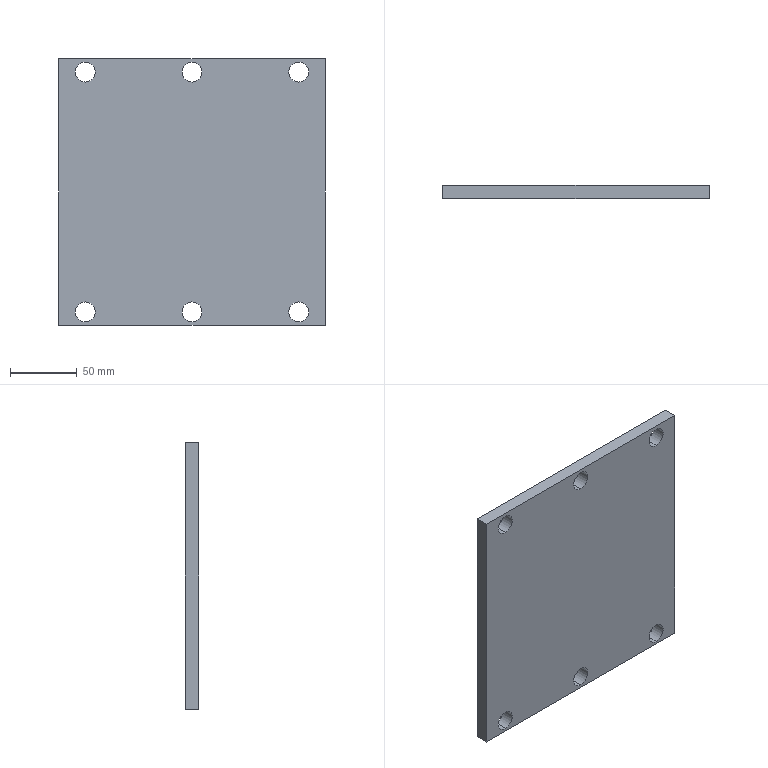Part | SolidWorks | features Extrusion 1, ICE 1, LPattern 1 | 1 solid | 18 faces | box 200 x 10 x 200 mm | volume 389397 mm3 | cylinder 12 | plane 6 | commonest cylinder face diameters 15 x12
STEP:
#1=CARTESIAN_POINT('',(80.,-5.,82.5));
#2=VERTEX_POINT('',#1);
#3=CARTESIAN_POINT('',(80.,-5.,97.5));
#4=VERTEX_POINT('',#3);
#5=CARTESIAN_POINT('',(80.,-5.,90.));
#6=DIRECTION('',(0.,1.,0.));
#7=DIRECTION('',(0.,0.,1.));
#8=AXIS2_PLACEMENT_3D('',#5,#6,#7);
#9=CIRCLE('',#8,7.5);
#10=EDGE_CURVE('',#2,#4,#9,.T.);
#11=ORIENTED_EDGE('',*,*,#10,.F.);
#12=CARTESIAN_POINT('',(80.,5.,82.5));
#13=VERTEX_POINT('',#12);
#14=CARTESIAN_POINT('',(80.,-5.,82.5));
#15=DIRECTION('',(0.,1.,0.));
#16=VECTOR('',#15,1000.);
#17=LINE('',#14,#16);
#18=EDGE_CURVE('',#2,#13,#17,.T.);
#19=ORIENTED_EDGE('',*,*,#18,.T.);
#20=CARTESIAN_POINT('',(80.,5.,97.5));
#21=VERTEX_POINT('',#20);
#22=CARTESIAN_POINT('',(80.,5.,90.));
#23=DIRECTION('',(0.,1.,0.));
#24=DIRECTION('',(0.,0.,1.));
#25=AXIS2_PLACEMENT_3D('',#22,#23,#24);
#26=CIRCLE('',#25,7.5);
#27=EDGE_CURVE('',#13,#21,#26,.T.);
#28=ORIENTED_EDGE('',*,*,#27,.T.);
#29=CARTESIAN_POINT('',(80.,-5.,97.5));
#30=DIRECTION('',(0.,1.,0.));
#31=VECTOR('',#30,1000.);
#32=LINE('',#29,#31);
#33=EDGE_CURVE('',#4,#21,#32,.T.);
#34=ORIENTED_EDGE('',*,*,#33,.F.);
#35=EDGE_LOOP('',(#11,#19,#28,#34));
#36=FACE_OUTER_BOUND('',#35,.T.);
#37=CARTESIAN_POINT('',(80.,-5.,90.));
#38=DIRECTION('',(0.,1.,0.));
#39=DIRECTION('',(0.,0.,1.));
#40=AXIS2_PLACEMENT_3D('',#37,#38,#39);
#41=CYLINDRICAL_SURFACE('',#40,7.5);
#42=ADVANCED_FACE('',(#36),#41,.F.);
#43=CARTESIAN_POINT('',(80.,-5.,-97.5));
#44=VERTEX_POINT('',#43);
#45=CARTESIAN_POINT('',(80.,-5.,-82.5));
#46=VERTEX_POINT('',#45);
#47=CARTESIAN_POINT('',(80.,-5.,-90.));
#48=DIRECTION('',(0.,1.,0.));
#49=DIRECTION('',(0.,0.,1.));
#50=AXIS2_PLACEMENT_3D('',#47,#48,#49);
#51=CIRCLE('',#50,7.5);
#52=EDGE_CURVE('',#44,#46,#51,.T.);
#53=ORIENTED_EDGE('',*,*,#52,.F.);
#54=CARTESIAN_POINT('',(80.,5.,-97.5));
#55=VERTEX_POINT('',#54);
#56=CARTESIAN_POINT('',(80.,-5.,-97.5));
#57=DIRECTION('',(0.,1.,0.));
#58=VECTOR('',#57,1000.);
#59=LINE('',#56,#58);
#60=EDGE_CURVE('',#44,#55,#59,.T.);
#61=ORIENTED_EDGE('',*,*,#60,.T.);
#62=CARTESIAN_POINT('',(80.,5.,-82.5));
#63=VERTEX_POINT('',#62);
#64=CARTESIAN_POINT('',(80.,5.,-90.));
#65=DIRECTION('',(0.,1.,0.));
#66=DIRECTION('',(0.,0.,1.));
#67=AXIS2_PLACEMENT_3D('',#64,#65,#66);
#68=CIRCLE('',#67,7.5);
#69=EDGE_CURVE('',#55,#63,#68,.T.);
#70=ORIENTED_EDGE('',*,*,#69,.T.);
#71=CARTESIAN_POINT('',(80.,-5.,-82.5));
#72=DIRECTION('',(0.,1.,0.));
#73=VECTOR('',#72,1000.);
#74=LINE('',#71,#73);
#75=EDGE_CURVE('',#46,#63,#74,.T.);
#76=ORIENTED_EDGE('',*,*,#75,.F.);
#77=EDGE_LOOP('',(#53,#61,#70,#76));
#78=FACE_OUTER_BOUND('',#77,.T.);
#79=CARTESIAN_POINT('',(80.,-5.,-90.));
#80=DIRECTION('',(0.,1.,0.));
#81=DIRECTION('',(0.,0.,1.));
#82=AXIS2_PLACEMENT_3D('',#79,#80,#81);
#83=CYLINDRICAL_SURFACE('',#82,7.5);
#84=ADVANCED_FACE('',(#78),#83,.F.);
#85=CARTESIAN_POINT('',(0.,-5.,-97.5));
#86=VERTEX_POINT('',#85);
#87=CARTESIAN_POINT('',(0.,-5.,-82.5));
#88=VERTEX_POINT('',#87);
#89=CARTESIAN_POINT('',(0.,-5.,-90.));
#90=DIRECTION('',(0.,1.,0.));
#91=DIRECTION('',(0.,0.,1.));
#92=AXIS2_PLACEMENT_3D('',#89,#90,#91);
#93=CIRCLE('',#92,7.5);
#94=EDGE_CURVE('',#86,#88,#93,.T.);
#95=ORIENTED_EDGE('',*,*,#94,.F.);
#96=CARTESIAN_POINT('',(0.,5.,-97.5));
#97=VERTEX_POINT('',#96);
#98=CARTESIAN_POINT('',(0.,-5.,-97.5));
#99=DIRECTION('',(0.,1.,0.));
#100=VECTOR('',#99,1000.);
#101=LINE('',#98,#100);
#102=EDGE_CURVE('',#86,#97,#101,.T.);
#103=ORIENTED_EDGE('',*,*,#102,.T.);
#104=CARTESIAN_POINT('',(0.,5.,-82.5));
#105=VERTEX_POINT('',#104);
#106=CARTESIAN_POINT('',(0.,5.,-90.));
#107=DIRECTION('',(0.,1.,0.));
#108=DIRECTION('',(0.,0.,1.));
#109=AXIS2_PLACEMENT_3D('',#106,#107,#108);
#110=CIRCLE('',#109,7.5);
#111=EDGE_CURVE('',#97,#105,#110,.T.);
#112=ORIENTED_EDGE('',*,*,#111,.T.);
#113=CARTESIAN_POINT('',(0.,-5.,-82.5));
#114=DIRECTION('',(0.,1.,0.));
#115=VECTOR('',#114,1000.);
#116=LINE('',#113,#115);
#117=EDGE_CURVE('',#88,#105,#116,.T.);
#118=ORIENTED_EDGE('',*,*,#117,.F.);
#119=EDGE_LOOP('',(#95,#103,#112,#118));
#120=FACE_OUTER_BOUND('',#119,.T.);
#121=CARTESIAN_POINT('',(0.,-5.,-90.));
#122=DIRECTION('',(0.,1.,0.));
#123=DIRECTION('',(0.,0.,1.));
#124=AXIS2_PLACEMENT_3D('',#121,#122,#123);
#125=CYLINDRICAL_SURFACE('',#124,7.5);
#126=ADVANCED_FACE('',(#120),#125,.F.);
#127=CARTESIAN_POINT('',(0.,-5.,82.5));
#128=VERTEX_POINT('',#127);
#129=CARTESIAN_POINT('',(0.,-5.,97.5));
#130=VERTEX_POINT('',#129);
#131=CARTESIAN_POINT('',(0.,-5.,90.));
#132=DIRECTION('',(0.,1.,0.));
#133=DIRECTION('',(0.,0.,1.));
#134=AXIS2_PLACEMENT_3D('',#131,#132,#133);
#135=CIRCLE('',#134,7.5);
#136=EDGE_CURVE('',#128,#130,#135,.T.);
#137=ORIENTED_EDGE('',*,*,#136,.F.);
#138=CARTESIAN_POINT('',(0.,5.,82.5));
#139=VERTEX_POINT('',#138);
#140=CARTESIAN_POINT('',(0.,-5.,82.5));
#141=DIRECTION('',(0.,1.,0.));
#142=VECTOR('',#141,1000.);
#143=LINE('',#140,#142);
#144=EDGE_CURVE('',#128,#139,#143,.T.);
#145=ORIENTED_EDGE('',*,*,#144,.T.);
#146=CARTESIAN_POINT('',(0.,5.,97.5));
#147=VERTEX_POINT('',#146);
#148=CARTESIAN_POINT('',(0.,5.,90.));
#149=DIRECTION('',(0.,1.,0.));
#150=DIRECTION('',(0.,0.,1.));
#151=AXIS2_PLACEMENT_3D('',#148,#149,#150);
#152=CIRCLE('',#151,7.5);
#153=EDGE_CURVE('',#139,#147,#152,.T.);
#154=ORIENTED_EDGE('',*,*,#153,.T.);
#155=CARTESIAN_POINT('',(0.,-5.,97.5));
#156=DIRECTION('',(0.,1.,0.));
#157=VECTOR('',#156,1000.);
#158=LINE('',#155,#157);
#159=EDGE_CURVE('',#130,#147,#158,.T.);
#160=ORIENTED_EDGE('',*,*,#159,.F.);
#161=EDGE_LOOP('',(#137,#145,#154,#160));
#162=FACE_OUTER_BOUND('',#161,.T.);
#163=CARTESIAN_POINT('',(0.,-5.,90.));
#164=DIRECTION('',(0.,1.,0.));
#165=DIRECTION('',(0.,0.,1.));
#166=AXIS2_PLACEMENT_3D('',#163,#164,#165);
#167=CYLINDRICAL_SURFACE('',#166,7.5);
#168=ADVANCED_FACE('',(#162),#167,.F.);
#169=CARTESIAN_POINT('',(-80.,-5.,-97.5));
#170=VERTEX_POINT('',#169);
#171=CARTESIAN_POINT('',(-80.,-5.,-82.5));
#172=VERTEX_POINT('',#171);
#173=CARTESIAN_POINT('',(-80.,-5.,-90.));
#174=DIRECTION('',(0.,1.,0.));
#175=DIRECTION('',(0.,0.,1.));
#176=AXIS2_PLACEMENT_3D('',#173,#174,#175);
#177=CIRCLE('',#176,7.5);
#178=EDGE_CURVE('',#170,#172,#177,.T.);
#179=ORIENTED_EDGE('',*,*,#178,.F.);
#180=CARTESIAN_POINT('',(-80.,5.,-97.5));
#181=VERTEX_POINT('',#180);
#182=CARTESIAN_POINT('',(-80.,-5.,-97.5));
#183=DIRECTION('',(0.,1.,0.));
#184=VECTOR('',#183,1000.);
#185=LINE('',#182,#184);
#186=EDGE_CURVE('',#170,#181,#185,.T.);
#187=ORIENTED_EDGE('',*,*,#186,.T.);
#188=CARTESIAN_POINT('',(-80.,5.,-82.5));
#189=VERTEX_POINT('',#188);
#190=CARTESIAN_POINT('',(-80.,5.,-90.));
#191=DIRECTION('',(0.,1.,0.));
#192=DIRECTION('',(0.,0.,1.));
#193=AXIS2_PLACEMENT_3D('',#190,#191,#192);
#194=CIRCLE('',#193,7.5);
#195=EDGE_CURVE('',#181,#189,#194,.T.);
#196=ORIENTED_EDGE('',*,*,#195,.T.);
#197=CARTESIAN_POINT('',(-80.,-5.,-82.5));
#198=DIRECTION('',(0.,1.,0.));
#199=VECTOR('',#198,1000.);
#200=LINE('',#197,#199);
#201=EDGE_CURVE('',#172,#189,#200,.T.);
#202=ORIENTED_EDGE('',*,*,#201,.F.);
#203=EDGE_LOOP('',(#179,#187,#196,#202));
#204=FACE_OUTER_BOUND('',#203,.T.);
#205=CARTESIAN_POINT('',(-80.,-5.,-90.));
#206=DIRECTION('',(0.,1.,0.));
#207=DIRECTION('',(0.,0.,1.));
#208=AXIS2_PLACEMENT_3D('',#205,#206,#207);
#209=CYLINDRICAL_SURFACE('',#208,7.5);
#210=ADVANCED_FACE('',(#204),#209,.F.);
#211=CARTESIAN_POINT('',(-80.,-5.,82.5));
#212=VERTEX_POINT('',#211);
#213=CARTESIAN_POINT('',(-80.,-5.,97.5));
#214=VERTEX_POINT('',#213);
#215=CARTESIAN_POINT('',(-80.,-5.,90.));
#216=DIRECTION('',(0.,1.,0.));
#217=DIRECTION('',(0.,0.,1.));
#218=AXIS2_PLACEMENT_3D('',#215,#216,#217);
#219=CIRCLE('',#218,7.5);
#220=EDGE_CURVE('',#212,#214,#219,.T.);
#221=ORIENTED_EDGE('',*,*,#220,.F.);
#222=CARTESIAN_POINT('',(-80.,5.,82.5));
#223=VERTEX_POINT('',#222);
#224=CARTESIAN_POINT('',(-80.,-5.,82.5));
#225=DIRECTION('',(0.,1.,0.));
#226=VECTOR('',#225,1000.);
#227=LINE('',#224,#226);
#228=EDGE_CURVE('',#212,#223,#227,.T.);
#229=ORIENTED_EDGE('',*,*,#228,.T.);
#230=CARTESIAN_POINT('',(-80.,5.,97.5));
#231=VERTEX_POINT('',#230);
#232=CARTESIAN_POINT('',(-80.,5.,90.));
#233=DIRECTION('',(0.,1.,0.));
#234=DIRECTION('',(0.,0.,1.));
#235=AXIS2_PLACEMENT_3D('',#232,#233,#234);
#236=CIRCLE('',#235,7.5);
#237=EDGE_CURVE('',#223,#231,#236,.T.);
#238=ORIENTED_EDGE('',*,*,#237,.T.);
#239=CARTESIAN_POINT('',(-80.,-5.,97.5));
#240=DIRECTION('',(0.,1.,0.));
#241=VECTOR('',#240,1000.);
#242=LINE('',#239,#241);
#243=EDGE_CURVE('',#214,#231,#242,.T.);
#244=ORIENTED_EDGE('',*,*,#243,.F.);
#245=EDGE_LOOP('',(#221,#229,#238,#244));
#246=FACE_OUTER_BOUND('',#245,.T.);
#247=CARTESIAN_POINT('',(-80.,-5.,90.));
#248=DIRECTION('',(0.,1.,0.));
#249=DIRECTION('',(0.,0.,1.));
#250=AXIS2_PLACEMENT_3D('',#247,#248,#249);
#251=CYLINDRICAL_SURFACE('',#250,7.5);
#252=ADVANCED_FACE('',(#246),#251,.F.);
#253=ORIENTED_EDGE('',*,*,#228,.F.);
#254=CARTESIAN_POINT('',(-80.,-5.,90.));
#255=DIRECTION('',(0.,1.,0.));
#256=DIRECTION('',(0.,0.,1.));
#257=AXIS2_PLACEMENT_3D('',#254,#255,#256);
#258=CIRCLE('',#257,7.5);
#259=EDGE_CURVE('',#214,#212,#258,.T.);
#260=ORIENTED_EDGE('',*,*,#259,.F.);
#261=ORIENTED_EDGE('',*,*,#243,.T.);
#262=CARTESIAN_POINT('',(-80.,5.,90.));
#263=DIRECTION('',(0.,1.,0.));
#264=DIRECTION('',(0.,0.,1.));
#265=AXIS2_PLACEMENT_3D('',#262,#263,#264);
#266=CIRCLE('',#265,7.5);
#267=EDGE_CURVE('',#231,#223,#266,.T.);
#268=ORIENTED_EDGE('',*,*,#267,.T.);
#269=EDGE_LOOP('',(#253,#260,#261,#268));
#270=FACE_OUTER_BOUND('',#269,.T.);
#271=CARTESIAN_POINT('',(-80.,-5.,90.));
#272=DIRECTION('',(0.,1.,0.));
#273=DIRECTION('',(0.,0.,1.));
#274=AXIS2_PLACEMENT_3D('',#271,#272,#273);
#275=CYLINDRICAL_SURFACE('',#274,7.5);
#276=ADVANCED_FACE('',(#270),#275,.F.);
#277=ORIENTED_EDGE('',*,*,#186,.F.);
#278=CARTESIAN_POINT('',(-80.,-5.,-90.));
#279=DIRECTION('',(0.,1.,0.));
#280=DIRECTION('',(0.,0.,1.));
#281=AXIS2_PLACEMENT_3D('',#278,#279,#280);
#282=CIRCLE('',#281,7.5);
#283=EDGE_CURVE('',#172,#170,#282,.T.);
#284=ORIENTED_EDGE('',*,*,#283,.F.);
#285=ORIENTED_EDGE('',*,*,#201,.T.);
#286=CARTESIAN_POINT('',(-80.,5.,-90.));
#287=DIRECTION('',(0.,1.,0.));
#288=DIRECTION('',(0.,0.,1.));
#289=AXIS2_PLACEMENT_3D('',#286,#287,#288);
#290=CIRCLE('',#289,7.5);
#291=EDGE_CURVE('',#189,#181,#290,.T.);
#292=ORIENTED_EDGE('',*,*,#291,.T.);
#293=EDGE_LOOP('',(#277,#284,#285,#292));
#294=FACE_OUTER_BOUND('',#293,.T.);
#295=CARTESIAN_POINT('',(-80.,-5.,-90.));
#296=DIRECTION('',(0.,1.,0.));
#297=DIRECTION('',(0.,0.,1.));
#298=AXIS2_PLACEMENT_3D('',#295,#296,#297);
#299=CYLINDRICAL_SURFACE('',#298,7.5);
#300=ADVANCED_FACE('',(#294),#299,.F.);
#301=ORIENTED_EDGE('',*,*,#144,.F.);
#302=CARTESIAN_POINT('',(0.,-5.,90.));
#303=DIRECTION('',(0.,1.,0.));
#304=DIRECTION('',(0.,0.,1.));
#305=AXIS2_PLACEMENT_3D('',#302,#303,#304);
#306=CIRCLE('',#305,7.5);
#307=EDGE_CURVE('',#130,#128,#306,.T.);
#308=ORIENTED_EDGE('',*,*,#307,.F.);
#309=ORIENTED_EDGE('',*,*,#159,.T.);
#310=CARTESIAN_POINT('',(0.,5.,90.));
#311=DIRECTION('',(0.,1.,0.));
#312=DIRECTION('',(0.,0.,1.));
#313=AXIS2_PLACEMENT_3D('',#310,#311,#312);
#314=CIRCLE('',#313,7.5);
#315=EDGE_CURVE('',#147,#139,#314,.T.);
#316=ORIENTED_EDGE('',*,*,#315,.T.);
#317=EDGE_LOOP('',(#301,#308,#309,#316));
#318=FACE_OUTER_BOUND('',#317,.T.);
#319=CARTESIAN_POINT('',(0.,-5.,90.));
#320=DIRECTION('',(0.,1.,0.));
#321=DIRECTION('',(0.,0.,1.));
#322=AXIS2_PLACEMENT_3D('',#319,#320,#321);
#323=CYLINDRICAL_SURFACE('',#322,7.5);
#324=ADVANCED_FACE('',(#318),#323,.F.);
#325=ORIENTED_EDGE('',*,*,#102,.F.);
#326=CARTESIAN_POINT('',(0.,-5.,-90.));
#327=DIRECTION('',(0.,1.,0.));
#328=DIRECTION('',(0.,0.,1.));
#329=AXIS2_PLACEMENT_3D('',#326,#327,#328);
#330=CIRCLE('',#329,7.5);
#331=EDGE_CURVE('',#88,#86,#330,.T.);
#332=ORIENTED_EDGE('',*,*,#331,.F.);
#333=ORIENTED_EDGE('',*,*,#117,.T.);
#334=CARTESIAN_POINT('',(0.,5.,-90.));
#335=DIRECTION('',(0.,1.,0.));
#336=DIRECTION('',(0.,0.,1.));
#337=AXIS2_PLACEMENT_3D('',#334,#335,#336);
#338=CIRCLE('',#337,7.5);
#339=EDGE_CURVE('',#105,#97,#338,.T.);
#340=ORIENTED_EDGE('',*,*,#339,.T.);
#341=EDGE_LOOP('',(#325,#332,#333,#340));
#342=FACE_OUTER_BOUND('',#341,.T.);
#343=CARTESIAN_POINT('',(0.,-5.,-90.));
#344=DIRECTION('',(0.,1.,0.));
#345=DIRECTION('',(0.,0.,1.));
#346=AXIS2_PLACEMENT_3D('',#343,#344,#345);
#347=CYLINDRICAL_SURFACE('',#346,7.5);
#348=ADVANCED_FACE('',(#342),#347,.F.);
#349=CARTESIAN_POINT('',(100.,-5.,100.));
#350=VERTEX_POINT('',#349);
#351=CARTESIAN_POINT('',(100.,-5.,-100.));
#352=VERTEX_POINT('',#351);
#353=CARTESIAN_POINT('',(100.,-5.,-100.));
#354=DIRECTION('',(0.,0.,-1.));
#355=VECTOR('',#354,1000.);
#356=LINE('',#353,#355);
#357=EDGE_CURVE('',#350,#352,#356,.T.);
#358=ORIENTED_EDGE('',*,*,#357,.T.);
#359=CARTESIAN_POINT('',(100.,5.,-100.));
#360=VERTEX_POINT('',#359);
#361=CARTESIAN_POINT('',(100.,5.,-100.));
#362=DIRECTION('',(0.,-1.,0.));
#363=VECTOR('',#362,1000.);
#364=LINE('',#361,#363);
#365=EDGE_CURVE('',#360,#352,#364,.T.);
#366=ORIENTED_EDGE('',*,*,#365,.F.);
#367=CARTESIAN_POINT('',(100.,5.,100.));
#368=VERTEX_POINT('',#367);
#369=CARTESIAN_POINT('',(100.,5.,-100.));
#370=DIRECTION('',(0.,0.,-1.));
#371=VECTOR('',#370,1000.);
#372=LINE('',#369,#371);
#373=EDGE_CURVE('',#368,#360,#372,.T.);
#374=ORIENTED_EDGE('',*,*,#373,.F.);
#375=CARTESIAN_POINT('',(100.,5.,100.));
#376=DIRECTION('',(0.,-1.,0.));
#377=VECTOR('',#376,1000.);
#378=LINE('',#375,#377);
#379=EDGE_CURVE('',#368,#350,#378,.T.);
#380=ORIENTED_EDGE('',*,*,#379,.T.);
#381=EDGE_LOOP('',(#358,#366,#374,#380));
#382=FACE_OUTER_BOUND('',#381,.T.);
#383=CARTESIAN_POINT('',(100.,5.,-100.));
#384=DIRECTION('',(-1.,0.,0.));
#385=DIRECTION('',(0.,0.,1.));
#386=AXIS2_PLACEMENT_3D('',#383,#384,#385);
#387=PLANE('',#386);
#388=ADVANCED_FACE('',(#382),#387,.F.);
#389=CARTESIAN_POINT('',(-100.,-5.,-100.));
#390=VERTEX_POINT('',#389);
#391=CARTESIAN_POINT('',(-100.,-5.,-100.));
#392=DIRECTION('',(-1.,0.,0.));
#393=VECTOR('',#392,1000.);
#394=LINE('',#391,#393);
#395=EDGE_CURVE('',#352,#390,#394,.T.);
#396=ORIENTED_EDGE('',*,*,#395,.T.);
#397=CARTESIAN_POINT('',(-100.,5.,-100.));
#398=VERTEX_POINT('',#397);
#399=CARTESIAN_POINT('',(-100.,5.,-100.));
#400=DIRECTION('',(0.,-1.,0.));
#401=VECTOR('',#400,1000.);
#402=LINE('',#399,#401);
#403=EDGE_CURVE('',#398,#390,#402,.T.);
#404=ORIENTED_EDGE('',*,*,#403,.F.);
#405=CARTESIAN_POINT('',(-100.,5.,-100.));
#406=DIRECTION('',(-1.,0.,0.));
#407=VECTOR('',#406,1000.);
#408=LINE('',#405,#407);
#409=EDGE_CURVE('',#360,#398,#408,.T.);
#410=ORIENTED_EDGE('',*,*,#409,.F.);
#411=ORIENTED_EDGE('',*,*,#365,.T.);
#412=EDGE_LOOP('',(#396,#404,#410,#411));
#413=FACE_OUTER_BOUND('',#412,.T.);
#414=CARTESIAN_POINT('',(-100.,5.,-100.));
#415=DIRECTION('',(0.,0.,1.));
#416=DIRECTION('',(1.,0.,0.));
#417=AXIS2_PLACEMENT_3D('',#414,#415,#416);
#418=PLANE('',#417);
#419=ADVANCED_FACE('',(#413),#418,.F.);
#420=CARTESIAN_POINT('',(-100.,-5.,100.));
#421=VERTEX_POINT('',#420);
#422=CARTESIAN_POINT('',(-100.,-5.,-100.));
#423=DIRECTION('',(0.,0.,1.));
#424=VECTOR('',#423,1000.);
#425=LINE('',#422,#424);
#426=EDGE_CURVE('',#390,#421,#425,.T.);
#427=ORIENTED_EDGE('',*,*,#426,.T.);
#428=CARTESIAN_POINT('',(-100.,5.,100.));
#429=VERTEX_POINT('',#428);
#430=CARTESIAN_POINT('',(-100.,5.,100.));
#431=DIRECTION('',(0.,-1.,0.));
#432=VECTOR('',#431,1000.);
#433=LINE('',#430,#432);
#434=EDGE_CURVE('',#429,#421,#433,.T.);
#435=ORIENTED_EDGE('',*,*,#434,.F.);
#436=CARTESIAN_POINT('',(-100.,5.,-100.));
#437=DIRECTION('',(0.,0.,1.));
#438=VECTOR('',#437,1000.);
#439=LINE('',#436,#438);
#440=EDGE_CURVE('',#398,#429,#439,.T.);
#441=ORIENTED_EDGE('',*,*,#440,.F.);
#442=ORIENTED_EDGE('',*,*,#403,.T.);
#443=EDGE_LOOP('',(#427,#435,#441,#442));
#444=FACE_OUTER_BOUND('',#443,.T.);
#445=CARTESIAN_POINT('',(-100.,5.,-100.));
#446=DIRECTION('',(1.,0.,0.));
#447=DIRECTION('',(0.,0.,-1.));
#448=AXIS2_PLACEMENT_3D('',#445,#446,#447);
#449=PLANE('',#448);
#450=ADVANCED_FACE('',(#444),#449,.F.);
#451=CARTESIAN_POINT('',(-100.,-5.,100.));
#452=DIRECTION('',(1.,0.,0.));
#453=VECTOR('',#452,1000.);
#454=LINE('',#451,#453);
#455=EDGE_CURVE('',#421,#350,#454,.T.);
#456=ORIENTED_EDGE('',*,*,#455,.T.);
#457=ORIENTED_EDGE('',*,*,#379,.F.);
#458=CARTESIAN_POINT('',(-100.,5.,100.));
#459=DIRECTION('',(1.,0.,0.));
#460=VECTOR('',#459,1000.);
#461=LINE('',#458,#460);
#462=EDGE_CURVE('',#429,#368,#461,.T.);
#463=ORIENTED_EDGE('',*,*,#462,.F.);
#464=ORIENTED_EDGE('',*,*,#434,.T.);
#465=EDGE_LOOP('',(#456,#457,#463,#464));
#466=FACE_OUTER_BOUND('',#465,.T.);
#467=CARTESIAN_POINT('',(-100.,5.,100.));
#468=DIRECTION('',(0.,0.,-1.));
#469=DIRECTION('',(-1.,0.,0.));
#470=AXIS2_PLACEMENT_3D('',#467,#468,#469);
#471=PLANE('',#470);
#472=ADVANCED_FACE('',(#466),#471,.F.);
#473=CARTESIAN_POINT('',(80.,5.,90.));
#474=DIRECTION('',(0.,1.,0.));
#475=DIRECTION('',(0.,0.,1.));
#476=AXIS2_PLACEMENT_3D('',#473,#474,#475);
#477=CIRCLE('',#476,7.5);
#478=EDGE_CURVE('',#21,#13,#477,.T.);
#479=ORIENTED_EDGE('',*,*,#478,.F.);
#480=ORIENTED_EDGE('',*,*,#27,.F.);
#481=EDGE_LOOP('',(#479,#480));
#482=FACE_BOUND('',#481,.T.);
#483=CARTESIAN_POINT('',(80.,5.,-90.));
#484=DIRECTION('',(0.,1.,0.));
#485=DIRECTION('',(0.,0.,1.));
#486=AXIS2_PLACEMENT_3D('',#483,#484,#485);
#487=CIRCLE('',#486,7.5);
#488=EDGE_CURVE('',#63,#55,#487,.T.);
#489=ORIENTED_EDGE('',*,*,#488,.F.);
#490=ORIENTED_EDGE('',*,*,#69,.F.);
#491=EDGE_LOOP('',(#489,#490));
#492=FACE_BOUND('',#491,.T.);
#493=ORIENTED_EDGE('',*,*,#373,.T.);
#494=ORIENTED_EDGE('',*,*,#409,.T.);
#495=ORIENTED_EDGE('',*,*,#440,.T.);
#496=ORIENTED_EDGE('',*,*,#462,.T.);
#497=EDGE_LOOP('',(#493,#494,#495,#496));
#498=FACE_OUTER_BOUND('',#497,.T.);
#499=ORIENTED_EDGE('',*,*,#339,.F.);
#500=ORIENTED_EDGE('',*,*,#111,.F.);
#501=EDGE_LOOP('',(#499,#500));
#502=FACE_BOUND('',#501,.T.);
#503=ORIENTED_EDGE('',*,*,#315,.F.);
#504=ORIENTED_EDGE('',*,*,#153,.F.);
#505=EDGE_LOOP('',(#503,#504));
#506=FACE_BOUND('',#505,.T.);
#507=ORIENTED_EDGE('',*,*,#291,.F.);
#508=ORIENTED_EDGE('',*,*,#195,.F.);
#509=EDGE_LOOP('',(#507,#508));
#510=FACE_BOUND('',#509,.T.);
#511=ORIENTED_EDGE('',*,*,#267,.F.);
#512=ORIENTED_EDGE('',*,*,#237,.F.);
#513=EDGE_LOOP('',(#511,#512));
#514=FACE_BOUND('',#513,.T.);
#515=CARTESIAN_POINT('',(0.,5.,0.));
#516=DIRECTION('',(0.,1.,0.));
#517=DIRECTION('',(0.,0.,1.));
#518=AXIS2_PLACEMENT_3D('',#515,#516,#517);
#519=PLANE('',#518);
#520=ADVANCED_FACE('',(#482,#492,#498,#502,#506,#510,#514),#519,.T.);
#521=CARTESIAN_POINT('',(80.,-5.,90.));
#522=DIRECTION('',(0.,1.,0.));
#523=DIRECTION('',(0.,0.,1.));
#524=AXIS2_PLACEMENT_3D('',#521,#522,#523);
#525=CIRCLE('',#524,7.5);
#526=EDGE_CURVE('',#4,#2,#525,.T.);
#527=ORIENTED_EDGE('',*,*,#526,.T.);
#528=ORIENTED_EDGE('',*,*,#10,.T.);
#529=EDGE_LOOP('',(#527,#528));
#530=FACE_BOUND('',#529,.T.);
#531=CARTESIAN_POINT('',(80.,-5.,-90.));
#532=DIRECTION('',(0.,1.,0.));
#533=DIRECTION('',(0.,0.,1.));
#534=AXIS2_PLACEMENT_3D('',#531,#532,#533);
#535=CIRCLE('',#534,7.5);
#536=EDGE_CURVE('',#46,#44,#535,.T.);
#537=ORIENTED_EDGE('',*,*,#536,.T.);
#538=ORIENTED_EDGE('',*,*,#52,.T.);
#539=EDGE_LOOP('',(#537,#538));
#540=FACE_BOUND('',#539,.T.);
#541=ORIENTED_EDGE('',*,*,#357,.F.);
#542=ORIENTED_EDGE('',*,*,#455,.F.);
#543=ORIENTED_EDGE('',*,*,#426,.F.);
#544=ORIENTED_EDGE('',*,*,#395,.F.);
#545=EDGE_LOOP('',(#541,#542,#543,#544));
#546=FACE_OUTER_BOUND('',#545,.T.);
#547=ORIENTED_EDGE('',*,*,#331,.T.);
#548=ORIENTED_EDGE('',*,*,#94,.T.);
#549=EDGE_LOOP('',(#547,#548));
#550=FACE_BOUND('',#549,.T.);
#551=ORIENTED_EDGE('',*,*,#307,.T.);
#552=ORIENTED_EDGE('',*,*,#136,.T.);
#553=EDGE_LOOP('',(#551,#552));
#554=FACE_BOUND('',#553,.T.);
#555=ORIENTED_EDGE('',*,*,#283,.T.);
#556=ORIENTED_EDGE('',*,*,#178,.T.);
#557=EDGE_LOOP('',(#555,#556));
#558=FACE_BOUND('',#557,.T.);
#559=ORIENTED_EDGE('',*,*,#259,.T.);
#560=ORIENTED_EDGE('',*,*,#220,.T.);
#561=EDGE_LOOP('',(#559,#560));
#562=FACE_BOUND('',#561,.T.);
#563=CARTESIAN_POINT('',(0.,-5.,0.));
#564=DIRECTION('',(0.,1.,0.));
#565=DIRECTION('',(0.,0.,1.));
#566=AXIS2_PLACEMENT_3D('',#563,#564,#565);
#567=PLANE('',#566);
#568=ADVANCED_FACE('',(#530,#540,#546,#550,#554,#558,#562),#567,.F.);
#569=ORIENTED_EDGE('',*,*,#60,.F.);
#570=ORIENTED_EDGE('',*,*,#536,.F.);
#571=ORIENTED_EDGE('',*,*,#75,.T.);
#572=ORIENTED_EDGE('',*,*,#488,.T.);
#573=EDGE_LOOP('',(#569,#570,#571,#572));
#574=FACE_OUTER_BOUND('',#573,.T.);
#575=CARTESIAN_POINT('',(80.,-5.,-90.));
#576=DIRECTION('',(0.,1.,0.));
#577=DIRECTION('',(0.,0.,1.));
#578=AXIS2_PLACEMENT_3D('',#575,#576,#577);
#579=CYLINDRICAL_SURFACE('',#578,7.5);
#580=ADVANCED_FACE('',(#574),#579,.F.);
#581=ORIENTED_EDGE('',*,*,#18,.F.);
#582=ORIENTED_EDGE('',*,*,#526,.F.);
#583=ORIENTED_EDGE('',*,*,#33,.T.);
#584=ORIENTED_EDGE('',*,*,#478,.T.);
#585=EDGE_LOOP('',(#581,#582,#583,#584));
#586=FACE_OUTER_BOUND('',#585,.T.);
#587=CARTESIAN_POINT('',(80.,-5.,90.));
#588=DIRECTION('',(0.,1.,0.));
#589=DIRECTION('',(0.,0.,1.));
#590=AXIS2_PLACEMENT_3D('',#587,#588,#589);
#591=CYLINDRICAL_SURFACE('',#590,7.5);
#592=ADVANCED_FACE('',(#586),#591,.F.);
#593=CLOSED_SHELL('',(#42,#84,#126,#168,#210,#252,#276,#300,#324,#348,#388,#419,#450,#472,#520,#568,#580,#592));
#594=MANIFOLD_SOLID_BREP('',#593);
#595=CARTESIAN_POINT('',(0.,0.,0.));
#596=DIRECTION('',(0.,0.,1.));
#597=DIRECTION('',(1.,0.,0.));
#598=AXIS2_PLACEMENT_3D('',#595,#596,#597);
#599=(LENGTH_UNIT()NAMED_UNIT(*)SI_UNIT(.MILLI.,.METRE.));
#600=UNCERTAINTY_MEASURE_WITH_UNIT(LENGTH_MEASURE(0.00001),#599,'','');
#601=(NAMED_UNIT(*)PLANE_ANGLE_UNIT()SI_UNIT($,.RADIAN.));
#602=(NAMED_UNIT(*)SI_UNIT($,.STERADIAN.)SOLID_ANGLE_UNIT());
#603=(GEOMETRIC_REPRESENTATION_CONTEXT(3)GLOBAL_UNCERTAINTY_ASSIGNED_CONTEXT((#600))GLOBAL_UNIT_ASSIGNED_CONTEXT((#599,#601,#602))REPRESENTATION_CONTEXT('',''));
#604=ADVANCED_BREP_SHAPE_REPRESENTATION('',(#594,#598),#603);